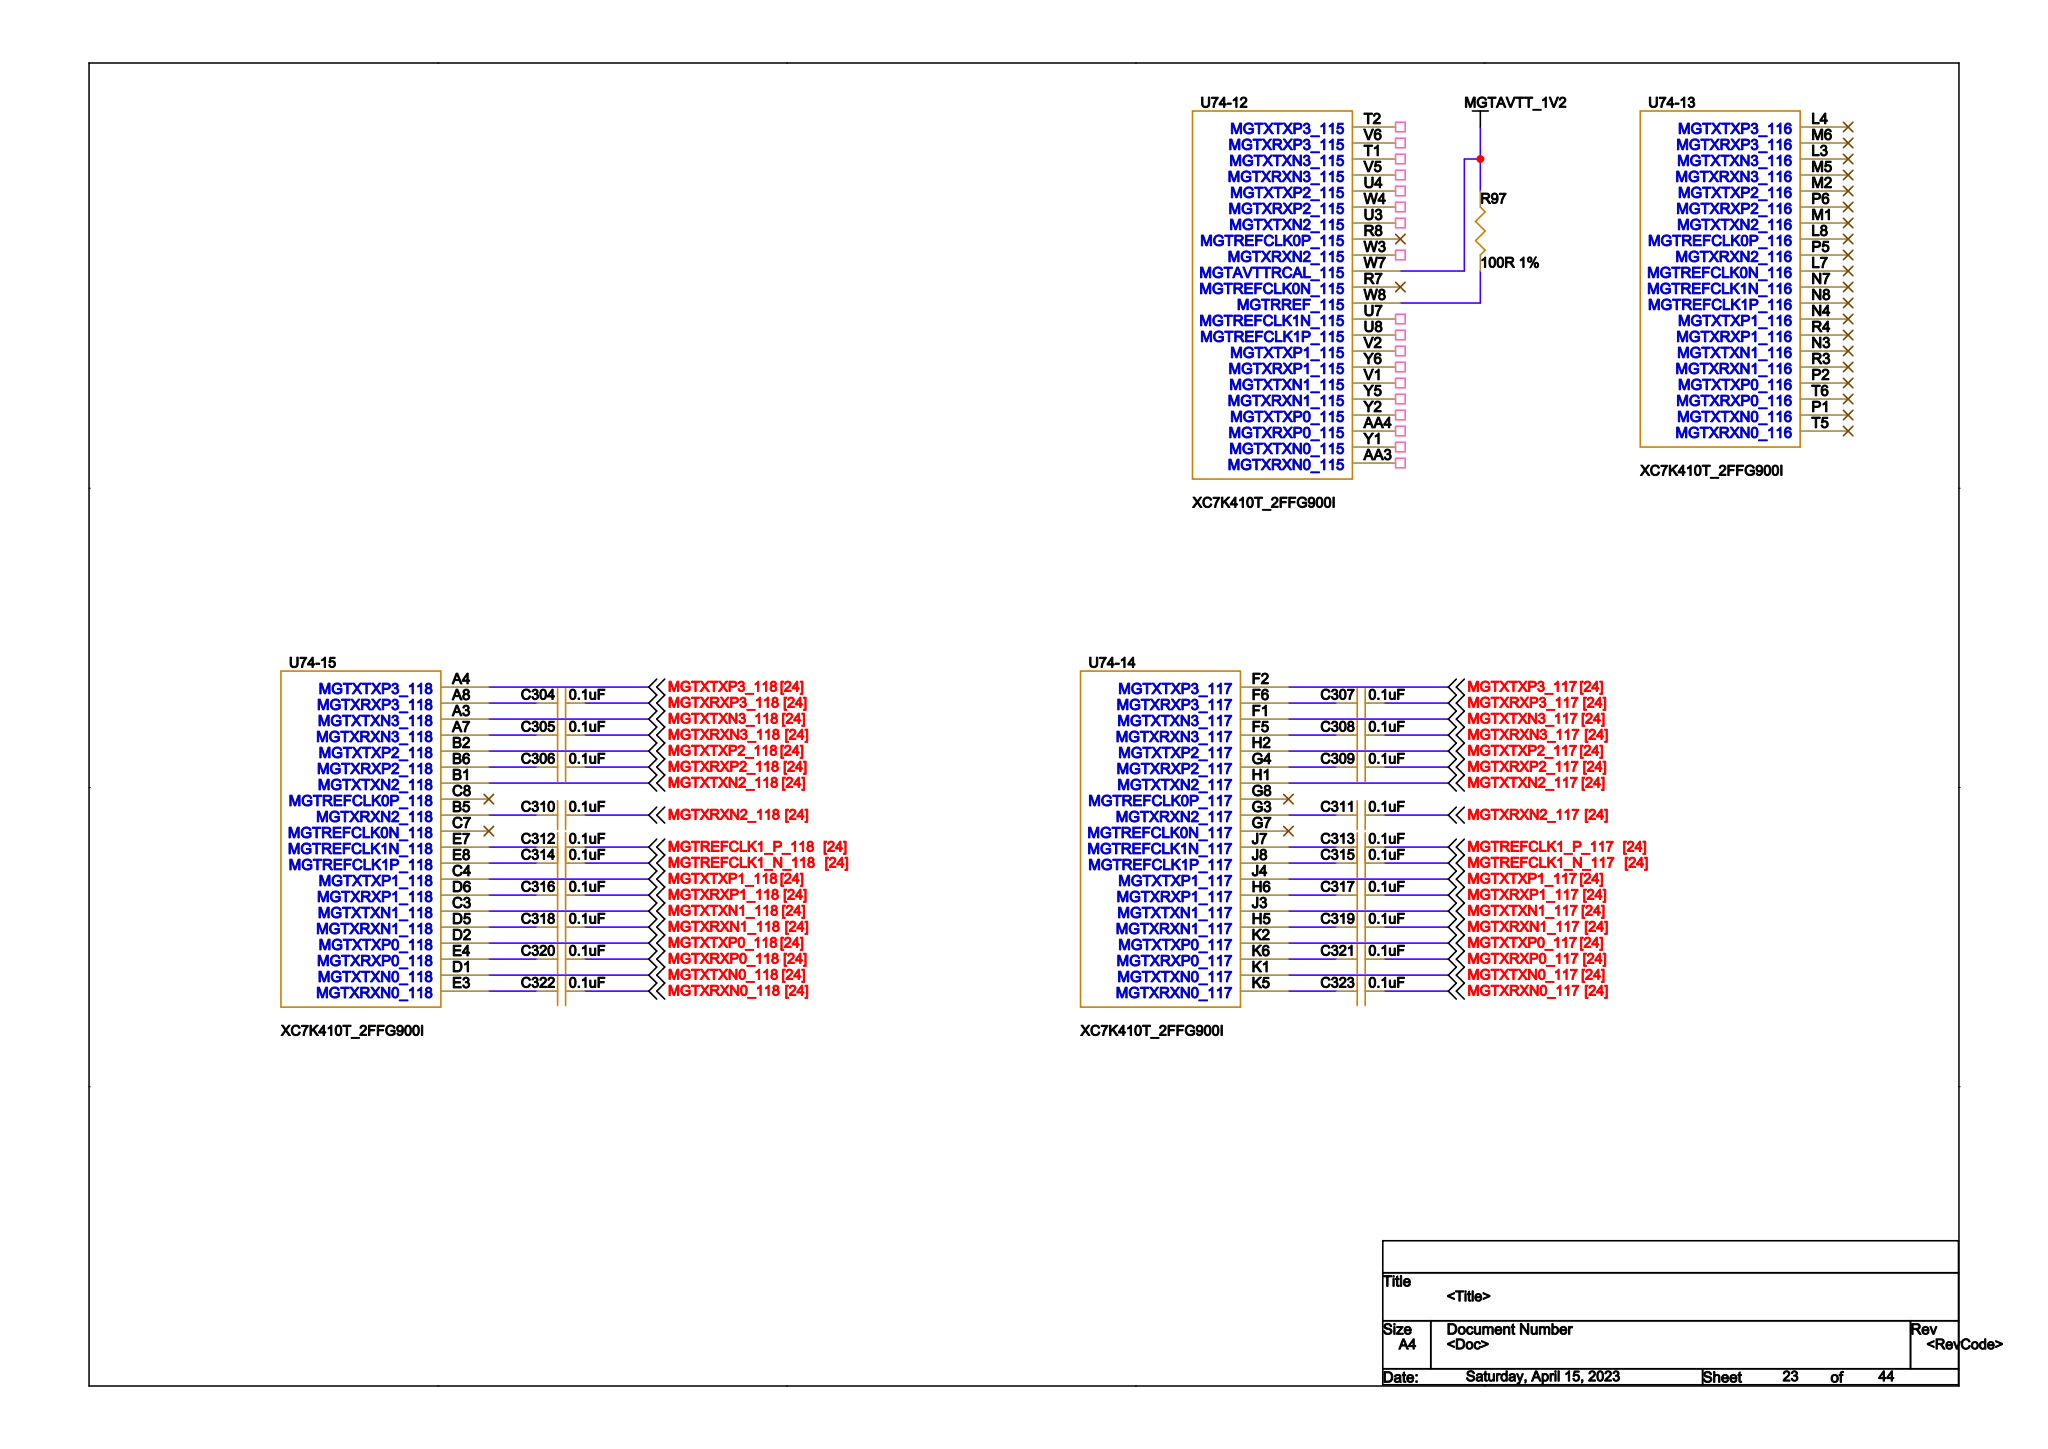Circuit board | Cadence Allegro | 1034 parts | 912 nets | one sheet of the schematic
Parts on this sheet (reference | value | footprint):
C304 | 0.1uF | C0402
C305 | 0.1uF | C0402
C306 | 0.1uF | C0402
C307 | 0.1uF | C0402
C308 | 0.1uF | C0402
C309 | 0.1uF | C0402
C310 | 0.1uF | C0402
C311 | 0.1uF | C0402
C312 | 0.1uF | C0402
C313 | 0.1uF | C0402
C314 | 0.1uF | C0402
C315 | 0.1uF | C0402
C316 | 0.1uF | C0402
C317 | 0.1uF | C0402
C318 | 0.1uF | C0402
C319 | 0.1uF | C0402
C320 | 0.1uF | C0402
C321 | 0.1uF | C0402
C322 | 0.1uF | C0402
C323 | 0.1uF | C0402
R97 | 100R 1% | R0402
Nets of these parts (net: part-pin ...):
MGTAVTT_1V2: R97-1
MGTXRXP3_118: C304-1
N13916328: C304-2
MGTXRXN3_118: C305-1
N13916342: C305-2
MGTXRXP2_118: C306-1
N13916344: C306-2
MGTXRXP3_117: C307-1
N13937445: C307-2
MGTXRXN3_117: C308-1
N13937489: C308-2
MGTXRXP2_117: C309-1
N13937533: C309-2
MGTXRXN2_118: C310-1
N13916330: C310-2
MGTXRXN2_117: C311-1
N13937577: C311-2
MGTREFCLK1_P_118: C312-1
N13916332: C312-2
MGTREFCLK1_P_117: C313-1
N13937609: C313-2
MGTREFCLK1_N_118: C314-1
N13916346: C314-2
MGTREFCLK1_N_117: C315-1
N13937641: C315-2
MGTXRXP1_118: C316-1
N13916334: C316-2
MGTXRXP1_117: C317-1
N13937685: C317-2
MGTXRXN1_118: C318-1
N13916348: C318-2
MGTXRXN1_117: C319-1
N13937729: C319-2
MGTXRXP0_118: C320-1
N13916338: C320-2
MGTXRXP0_117: C321-1
N13937773: C321-2
MGTXRXN0_118: C322-1
N13916350: C322-2
MGTXRXN0_117: C323-1
N13937817: C323-2
N251139: R97-2